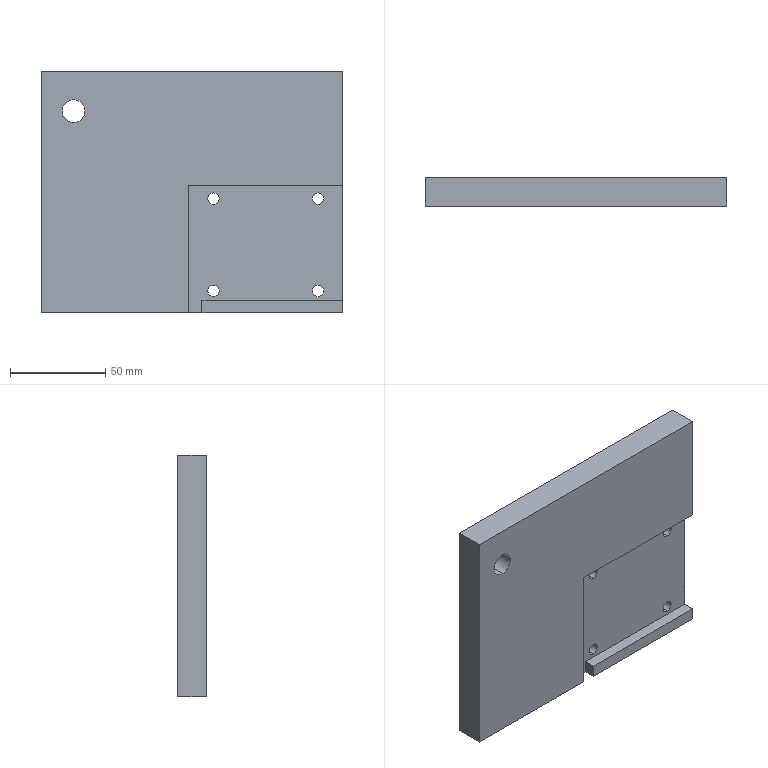Part | SolidWorks | features ICE 6, Extrusion 1, HoleWzd 1 | 1 solid | 34 faces | box 158.5 x 15 x 127 mm | volume 237591 mm3 | plane 16 | cylinder 14 | cone 4 | commonest cylinder face diameters 6 x8 5 x2 12 x2 20 x2
STEP:
#1=CARTESIAN_POINT('',(-38.25,9.498,24.5));
#2=VERTEX_POINT('',#1);
#3=CARTESIAN_POINT('',(-38.25,11.,27.));
#4=VERTEX_POINT('',#3);
#5=CARTESIAN_POINT('',(-38.25,11.,27.));
#6=DIRECTION('',(0.,0.515,0.8572));
#7=VECTOR('',#6,1000.);
#8=LINE('',#5,#7);
#9=EDGE_CURVE('',#2,#4,#8,.T.);
#10=ORIENTED_EDGE('',*,*,#9,.F.);
#11=CARTESIAN_POINT('',(-38.25,11.,22.));
#12=VERTEX_POINT('',#11);
#13=CARTESIAN_POINT('',(-38.25,11.,22.));
#14=DIRECTION('',(0.,0.515,-0.8572));
#15=VECTOR('',#14,1000.);
#16=LINE('',#13,#15);
#17=EDGE_CURVE('',#2,#12,#16,.T.);
#18=ORIENTED_EDGE('',*,*,#17,.T.);
#19=CARTESIAN_POINT('',(-38.25,11.,24.5));
#20=DIRECTION('',(0.,1.,0.));
#21=DIRECTION('',(0.,0.,1.));
#22=AXIS2_PLACEMENT_3D('',#19,#20,#21);
#23=CIRCLE('',#22,2.5);
#24=EDGE_CURVE('',#12,#4,#23,.T.);
#25=ORIENTED_EDGE('',*,*,#24,.T.);
#26=EDGE_LOOP('',(#10,#18,#25));
#27=FACE_OUTER_BOUND('',#26,.T.);
#28=CARTESIAN_POINT('',(-38.25,11.,24.5));
#29=DIRECTION('',(0.,1.,0.));
#30=DIRECTION('',(0.,0.,1.));
#31=AXIS2_PLACEMENT_3D('',#28,#29,#30);
#32=CONICAL_SURFACE('',#31,2.5,1.03);
#33=ADVANCED_FACE('',(#27),#32,.F.);
#34=CARTESIAN_POINT('',(-38.25,14.975,27.));
#35=VERTEX_POINT('',#34);
#36=CARTESIAN_POINT('',(-35.75,14.975,24.5));
#37=VERTEX_POINT('',#36);
#38=CARTESIAN_POINT('',(-38.25,14.975,24.5));
#39=DIRECTION('',(0.,1.,0.));
#40=DIRECTION('',(0.,0.,1.));
#41=AXIS2_PLACEMENT_3D('',#38,#39,#40);
#42=CIRCLE('',#41,2.5);
#43=EDGE_CURVE('',#35,#37,#42,.T.);
#44=ORIENTED_EDGE('',*,*,#43,.F.);
#45=CARTESIAN_POINT('',(-38.25,15.,27.025));
#46=VERTEX_POINT('',#45);
#47=CARTESIAN_POINT('',(-38.25,15.,27.025));
#48=DIRECTION('',(0.,0.7071,0.7071));
#49=VECTOR('',#48,1000.);
#50=LINE('',#47,#49);
#51=EDGE_CURVE('',#35,#46,#50,.T.);
#52=ORIENTED_EDGE('',*,*,#51,.T.);
#53=CARTESIAN_POINT('',(-35.725,15.,24.5));
#54=VERTEX_POINT('',#53);
#55=CARTESIAN_POINT('',(-38.25,15.,24.5));
#56=DIRECTION('',(0.,1.,0.));
#57=DIRECTION('',(0.,0.,1.));
#58=AXIS2_PLACEMENT_3D('',#55,#56,#57);
#59=CIRCLE('',#58,2.525);
#60=EDGE_CURVE('',#46,#54,#59,.T.);
#61=ORIENTED_EDGE('',*,*,#60,.T.);
#62=CARTESIAN_POINT('',(-38.25,12.475,24.5));
#63=DIRECTION('',(0.7071,0.7071,0.));
#64=VECTOR('',#63,1000.);
#65=LINE('',#62,#64);
#66=EDGE_CURVE('',#37,#54,#65,.T.);
#67=ORIENTED_EDGE('',*,*,#66,.F.);
#68=EDGE_LOOP('',(#44,#52,#61,#67));
#69=FACE_OUTER_BOUND('',#68,.T.);
#70=CARTESIAN_POINT('',(-38.25,15.,24.5));
#71=DIRECTION('',(0.,1.,0.));
#72=DIRECTION('',(0.,0.,1.));
#73=AXIS2_PLACEMENT_3D('',#70,#71,#72);
#74=CONICAL_SURFACE('',#73,2.525,0.7854);
#75=ADVANCED_FACE('',(#69),#74,.F.);
#76=ORIENTED_EDGE('',*,*,#24,.F.);
#77=CARTESIAN_POINT('',(-38.25,12.,22.));
#78=VERTEX_POINT('',#77);
#79=CARTESIAN_POINT('',(-38.25,15.,22.));
#80=DIRECTION('',(0.,1.,0.));
#81=VECTOR('',#80,1000.);
#82=LINE('',#79,#81);
#83=EDGE_CURVE('',#12,#78,#82,.T.);
#84=ORIENTED_EDGE('',*,*,#83,.T.);
#85=CARTESIAN_POINT('',(-38.25,14.975,22.));
#86=VERTEX_POINT('',#85);
#87=CARTESIAN_POINT('',(-38.25,15.,22.));
#88=DIRECTION('',(0.,-1.,0.));
#89=VECTOR('',#88,1000.);
#90=LINE('',#87,#89);
#91=EDGE_CURVE('',#86,#78,#90,.T.);
#92=ORIENTED_EDGE('',*,*,#91,.F.);
#93=CARTESIAN_POINT('',(-38.25,14.975,24.5));
#94=DIRECTION('',(0.,1.,0.));
#95=DIRECTION('',(0.,0.,1.));
#96=AXIS2_PLACEMENT_3D('',#93,#94,#95);
#97=CIRCLE('',#96,2.5);
#98=EDGE_CURVE('',#86,#35,#97,.T.);
#99=ORIENTED_EDGE('',*,*,#98,.T.);
#100=CARTESIAN_POINT('',(-38.25,15.,27.));
#101=DIRECTION('',(0.,1.,0.));
#102=VECTOR('',#101,1000.);
#103=LINE('',#100,#102);
#104=EDGE_CURVE('',#4,#35,#103,.T.);
#105=ORIENTED_EDGE('',*,*,#104,.F.);
#106=EDGE_LOOP('',(#76,#84,#92,#99,#105));
#107=FACE_OUTER_BOUND('',#106,.T.);
#108=CARTESIAN_POINT('',(-38.25,15.,24.5));
#109=DIRECTION('',(0.,1.,0.));
#110=DIRECTION('',(0.,0.,1.));
#111=AXIS2_PLACEMENT_3D('',#108,#109,#110);
#112=CYLINDRICAL_SURFACE('',#111,2.5);
#113=ADVANCED_FACE('',(#107),#112,.F.);
#114=CARTESIAN_POINT('',(-62.25,0.,36.5));
#115=VERTEX_POINT('',#114);
#116=CARTESIAN_POINT('',(-62.25,0.,48.5));
#117=VERTEX_POINT('',#116);
#118=CARTESIAN_POINT('',(-62.25,0.,42.5));
#119=DIRECTION('',(0.,1.,0.));
#120=DIRECTION('',(0.,0.,1.));
#121=AXIS2_PLACEMENT_3D('',#118,#119,#120);
#122=CIRCLE('',#121,6.);
#123=EDGE_CURVE('',#115,#117,#122,.T.);
#124=ORIENTED_EDGE('',*,*,#123,.F.);
#125=CARTESIAN_POINT('',(-62.25,9.,36.5));
#126=VERTEX_POINT('',#125);
#127=CARTESIAN_POINT('',(-62.25,0.,36.5));
#128=DIRECTION('',(0.,1.,0.));
#129=VECTOR('',#128,1000.);
#130=LINE('',#127,#129);
#131=EDGE_CURVE('',#115,#126,#130,.T.);
#132=ORIENTED_EDGE('',*,*,#131,.T.);
#133=CARTESIAN_POINT('',(-62.25,9.,48.5));
#134=VERTEX_POINT('',#133);
#135=CARTESIAN_POINT('',(-62.25,9.,42.5));
#136=DIRECTION('',(0.,1.,0.));
#137=DIRECTION('',(0.,0.,1.));
#138=AXIS2_PLACEMENT_3D('',#135,#136,#137);
#139=CIRCLE('',#138,6.);
#140=EDGE_CURVE('',#126,#134,#139,.T.);
#141=ORIENTED_EDGE('',*,*,#140,.T.);
#142=CARTESIAN_POINT('',(-62.25,0.,48.5));
#143=DIRECTION('',(0.,1.,0.));
#144=VECTOR('',#143,1000.);
#145=LINE('',#142,#144);
#146=EDGE_CURVE('',#117,#134,#145,.T.);
#147=ORIENTED_EDGE('',*,*,#146,.F.);
#148=EDGE_LOOP('',(#124,#132,#141,#147));
#149=FACE_OUTER_BOUND('',#148,.T.);
#150=CARTESIAN_POINT('',(-62.25,0.,42.5));
#151=DIRECTION('',(0.,1.,0.));
#152=DIRECTION('',(0.,0.,1.));
#153=AXIS2_PLACEMENT_3D('',#150,#151,#152);
#154=CYLINDRICAL_SURFACE('',#153,6.);
#155=ADVANCED_FACE('',(#149),#154,.F.);
#156=CARTESIAN_POINT('',(-62.25,9.,32.5));
#157=VERTEX_POINT('',#156);
#158=CARTESIAN_POINT('',(-62.25,9.,52.5));
#159=VERTEX_POINT('',#158);
#160=CARTESIAN_POINT('',(-62.25,9.,42.5));
#161=DIRECTION('',(0.,1.,0.));
#162=DIRECTION('',(0.,0.,1.));
#163=AXIS2_PLACEMENT_3D('',#160,#161,#162);
#164=CIRCLE('',#163,10.);
#165=EDGE_CURVE('',#157,#159,#164,.T.);
#166=ORIENTED_EDGE('',*,*,#165,.F.);
#167=CARTESIAN_POINT('',(-62.25,15.,32.5));
#168=VERTEX_POINT('',#167);
#169=CARTESIAN_POINT('',(-62.25,9.,32.5));
#170=DIRECTION('',(0.,1.,0.));
#171=VECTOR('',#170,1000.);
#172=LINE('',#169,#171);
#173=EDGE_CURVE('',#157,#168,#172,.T.);
#174=ORIENTED_EDGE('',*,*,#173,.T.);
#175=CARTESIAN_POINT('',(-62.25,15.,52.5));
#176=VERTEX_POINT('',#175);
#177=CARTESIAN_POINT('',(-62.25,15.,42.5));
#178=DIRECTION('',(0.,1.,0.));
#179=DIRECTION('',(0.,0.,1.));
#180=AXIS2_PLACEMENT_3D('',#177,#178,#179);
#181=CIRCLE('',#180,10.);
#182=EDGE_CURVE('',#168,#176,#181,.T.);
#183=ORIENTED_EDGE('',*,*,#182,.T.);
#184=CARTESIAN_POINT('',(-62.25,9.,52.5));
#185=DIRECTION('',(0.,1.,0.));
#186=VECTOR('',#185,1000.);
#187=LINE('',#184,#186);
#188=EDGE_CURVE('',#159,#176,#187,.T.);
#189=ORIENTED_EDGE('',*,*,#188,.F.);
#190=EDGE_LOOP('',(#166,#174,#183,#189));
#191=FACE_OUTER_BOUND('',#190,.T.);
#192=CARTESIAN_POINT('',(-62.25,9.,42.5));
#193=DIRECTION('',(0.,1.,0.));
#194=DIRECTION('',(0.,0.,1.));
#195=AXIS2_PLACEMENT_3D('',#192,#193,#194);
#196=CYLINDRICAL_SURFACE('',#195,10.);
#197=ADVANCED_FACE('',(#191),#196,.F.);
#198=CARTESIAN_POINT('',(11.25,6.,-0.5));
#199=VERTEX_POINT('',#198);
#200=CARTESIAN_POINT('',(11.25,6.,-6.5));
#201=VERTEX_POINT('',#200);
#202=CARTESIAN_POINT('',(11.25,6.,-3.5));
#203=DIRECTION('',(0.,-1.,0.));
#204=DIRECTION('',(0.,0.,-1.));
#205=AXIS2_PLACEMENT_3D('',#202,#203,#204);
#206=CIRCLE('',#205,3.);
#207=EDGE_CURVE('',#199,#201,#206,.T.);
#208=ORIENTED_EDGE('',*,*,#207,.T.);
#209=CARTESIAN_POINT('',(11.25,12.,-6.5));
#210=VERTEX_POINT('',#209);
#211=CARTESIAN_POINT('',(11.25,0.,-6.5));
#212=DIRECTION('',(0.,1.,0.));
#213=VECTOR('',#212,1000.);
#214=LINE('',#211,#213);
#215=EDGE_CURVE('',#201,#210,#214,.T.);
#216=ORIENTED_EDGE('',*,*,#215,.T.);
#217=CARTESIAN_POINT('',(11.25,12.,-0.5));
#218=VERTEX_POINT('',#217);
#219=CARTESIAN_POINT('',(11.25,12.,-3.5));
#220=DIRECTION('',(0.,-1.,0.));
#221=DIRECTION('',(0.,0.,-1.));
#222=AXIS2_PLACEMENT_3D('',#219,#220,#221);
#223=CIRCLE('',#222,3.);
#224=EDGE_CURVE('',#218,#210,#223,.T.);
#225=ORIENTED_EDGE('',*,*,#224,.F.);
#226=CARTESIAN_POINT('',(11.25,0.,-0.5));
#227=DIRECTION('',(0.,1.,0.));
#228=VECTOR('',#227,1000.);
#229=LINE('',#226,#228);
#230=EDGE_CURVE('',#199,#218,#229,.T.);
#231=ORIENTED_EDGE('',*,*,#230,.F.);
#232=EDGE_LOOP('',(#208,#216,#225,#231));
#233=FACE_OUTER_BOUND('',#232,.T.);
#234=CARTESIAN_POINT('',(11.25,0.,-3.5));
#235=DIRECTION('',(0.,1.,0.));
#236=DIRECTION('',(0.,0.,1.));
#237=AXIS2_PLACEMENT_3D('',#234,#235,#236);
#238=CYLINDRICAL_SURFACE('',#237,3.);
#239=ADVANCED_FACE('',(#233),#238,.F.);
#240=CARTESIAN_POINT('',(66.25,6.,-0.5));
#241=VERTEX_POINT('',#240);
#242=CARTESIAN_POINT('',(66.25,6.,-6.5));
#243=VERTEX_POINT('',#242);
#244=CARTESIAN_POINT('',(66.25,6.,-3.5));
#245=DIRECTION('',(0.,-1.,0.));
#246=DIRECTION('',(0.,0.,-1.));
#247=AXIS2_PLACEMENT_3D('',#244,#245,#246);
#248=CIRCLE('',#247,3.);
#249=EDGE_CURVE('',#241,#243,#248,.T.);
#250=ORIENTED_EDGE('',*,*,#249,.T.);
#251=CARTESIAN_POINT('',(66.25,12.,-6.5));
#252=VERTEX_POINT('',#251);
#253=CARTESIAN_POINT('',(66.25,0.,-6.5));
#254=DIRECTION('',(0.,1.,0.));
#255=VECTOR('',#254,1000.);
#256=LINE('',#253,#255);
#257=EDGE_CURVE('',#243,#252,#256,.T.);
#258=ORIENTED_EDGE('',*,*,#257,.T.);
#259=CARTESIAN_POINT('',(66.25,12.,-0.5));
#260=VERTEX_POINT('',#259);
#261=CARTESIAN_POINT('',(66.25,12.,-3.5));
#262=DIRECTION('',(0.,-1.,0.));
#263=DIRECTION('',(0.,0.,-1.));
#264=AXIS2_PLACEMENT_3D('',#261,#262,#263);
#265=CIRCLE('',#264,3.);
#266=EDGE_CURVE('',#260,#252,#265,.T.);
#267=ORIENTED_EDGE('',*,*,#266,.F.);
#268=CARTESIAN_POINT('',(66.25,0.,-0.5));
#269=DIRECTION('',(0.,1.,0.));
#270=VECTOR('',#269,1000.);
#271=LINE('',#268,#270);
#272=EDGE_CURVE('',#241,#260,#271,.T.);
#273=ORIENTED_EDGE('',*,*,#272,.F.);
#274=EDGE_LOOP('',(#250,#258,#267,#273));
#275=FACE_OUTER_BOUND('',#274,.T.);
#276=CARTESIAN_POINT('',(66.25,0.,-3.5));
#277=DIRECTION('',(0.,1.,0.));
#278=DIRECTION('',(0.,0.,1.));
#279=AXIS2_PLACEMENT_3D('',#276,#277,#278);
#280=CYLINDRICAL_SURFACE('',#279,3.);
#281=ADVANCED_FACE('',(#275),#280,.F.);
#282=CARTESIAN_POINT('',(66.25,6.,-49.));
#283=VERTEX_POINT('',#282);
#284=CARTESIAN_POINT('',(66.25,6.,-55.));
#285=VERTEX_POINT('',#284);
#286=CARTESIAN_POINT('',(66.25,6.,-52.));
#287=DIRECTION('',(0.,-1.,0.));
#288=DIRECTION('',(0.,0.,-1.));
#289=AXIS2_PLACEMENT_3D('',#286,#287,#288);
#290=CIRCLE('',#289,3.);
#291=EDGE_CURVE('',#283,#285,#290,.T.);
#292=ORIENTED_EDGE('',*,*,#291,.T.);
#293=CARTESIAN_POINT('',(66.25,12.,-55.));
#294=VERTEX_POINT('',#293);
#295=CARTESIAN_POINT('',(66.25,0.,-55.));
#296=DIRECTION('',(0.,1.,0.));
#297=VECTOR('',#296,1000.);
#298=LINE('',#295,#297);
#299=EDGE_CURVE('',#285,#294,#298,.T.);
#300=ORIENTED_EDGE('',*,*,#299,.T.);
#301=CARTESIAN_POINT('',(66.25,12.,-49.));
#302=VERTEX_POINT('',#301);
#303=CARTESIAN_POINT('',(66.25,12.,-52.));
#304=DIRECTION('',(0.,-1.,0.));
#305=DIRECTION('',(0.,0.,-1.));
#306=AXIS2_PLACEMENT_3D('',#303,#304,#305);
#307=CIRCLE('',#306,3.);
#308=EDGE_CURVE('',#302,#294,#307,.T.);
#309=ORIENTED_EDGE('',*,*,#308,.F.);
#310=CARTESIAN_POINT('',(66.25,0.,-49.));
#311=DIRECTION('',(0.,1.,0.));
#312=VECTOR('',#311,1000.);
#313=LINE('',#310,#312);
#314=EDGE_CURVE('',#283,#302,#313,.T.);
#315=ORIENTED_EDGE('',*,*,#314,.F.);
#316=EDGE_LOOP('',(#292,#300,#309,#315));
#317=FACE_OUTER_BOUND('',#316,.T.);
#318=CARTESIAN_POINT('',(66.25,0.,-52.));
#319=DIRECTION('',(0.,1.,0.));
#320=DIRECTION('',(0.,0.,1.));
#321=AXIS2_PLACEMENT_3D('',#318,#319,#320);
#322=CYLINDRICAL_SURFACE('',#321,3.);
#323=ADVANCED_FACE('',(#317),#322,.F.);
#324=CARTESIAN_POINT('',(11.25,6.,-49.));
#325=VERTEX_POINT('',#324);
#326=CARTESIAN_POINT('',(11.25,6.,-55.));
#327=VERTEX_POINT('',#326);
#328=CARTESIAN_POINT('',(11.25,6.,-52.));
#329=DIRECTION('',(0.,-1.,0.));
#330=DIRECTION('',(0.,0.,-1.));
#331=AXIS2_PLACEMENT_3D('',#328,#329,#330);
#332=CIRCLE('',#331,3.);
#333=EDGE_CURVE('',#325,#327,#332,.T.);
#334=ORIENTED_EDGE('',*,*,#333,.T.);
#335=CARTESIAN_POINT('',(11.25,12.,-55.));
#336=VERTEX_POINT('',#335);
#337=CARTESIAN_POINT('',(11.25,0.,-55.));
#338=DIRECTION('',(0.,1.,0.));
#339=VECTOR('',#338,1000.);
#340=LINE('',#337,#339);
#341=EDGE_CURVE('',#327,#336,#340,.T.);
#342=ORIENTED_EDGE('',*,*,#341,.T.);
#343=CARTESIAN_POINT('',(11.25,12.,-49.));
#344=VERTEX_POINT('',#343);
#345=CARTESIAN_POINT('',(11.25,12.,-52.));
#346=DIRECTION('',(0.,-1.,0.));
#347=DIRECTION('',(0.,0.,-1.));
#348=AXIS2_PLACEMENT_3D('',#345,#346,#347);
#349=CIRCLE('',#348,3.);
#350=EDGE_CURVE('',#344,#336,#349,.T.);
#351=ORIENTED_EDGE('',*,*,#350,.F.);
#352=CARTESIAN_POINT('',(11.25,0.,-49.));
#353=DIRECTION('',(0.,1.,0.));
#354=VECTOR('',#353,1000.);
#355=LINE('',#352,#354);
#356=EDGE_CURVE('',#325,#344,#355,.T.);
#357=ORIENTED_EDGE('',*,*,#356,.F.);
#358=EDGE_LOOP('',(#334,#342,#351,#357));
#359=FACE_OUTER_BOUND('',#358,.T.);
#360=CARTESIAN_POINT('',(11.25,0.,-52.));
#361=DIRECTION('',(0.,1.,0.));
#362=DIRECTION('',(0.,0.,1.));
#363=AXIS2_PLACEMENT_3D('',#360,#361,#362);
#364=CYLINDRICAL_SURFACE('',#363,3.);
#365=ADVANCED_FACE('',(#359),#364,.F.);
#366=CARTESIAN_POINT('',(-62.25,0.,42.5));
#367=DIRECTION('',(0.,1.,0.));
#368=DIRECTION('',(0.,0.,1.));
#369=AXIS2_PLACEMENT_3D('',#366,#367,#368);
#370=CIRCLE('',#369,6.);
#371=EDGE_CURVE('',#117,#115,#370,.T.);
#372=ORIENTED_EDGE('',*,*,#371,.T.);
#373=ORIENTED_EDGE('',*,*,#123,.T.);
#374=EDGE_LOOP('',(#372,#373));
#375=FACE_BOUND('',#374,.T.);
#376=CARTESIAN_POINT('',(-1.75,0.,-63.5));
#377=VERTEX_POINT('',#376);
#378=CARTESIAN_POINT('',(-79.25,0.,-63.5));
#379=VERTEX_POINT('',#378);
#380=CARTESIAN_POINT('',(-79.25,0.,-63.5));
#381=DIRECTION('',(-1.,0.,0.));
#382=VECTOR('',#381,1000.);
#383=LINE('',#380,#382);
#384=EDGE_CURVE('',#377,#379,#383,.T.);
#385=ORIENTED_EDGE('',*,*,#384,.F.);
#386=CARTESIAN_POINT('',(-1.75,0.,3.5));
#387=VERTEX_POINT('',#386);
#388=CARTESIAN_POINT('',(-1.75,0.,-57.));
#389=DIRECTION('',(0.,0.,-1.));
#390=VECTOR('',#389,1000.);
#391=LINE('',#388,#390);
#392=EDGE_CURVE('',#387,#377,#391,.T.);
#393=ORIENTED_EDGE('',*,*,#392,.F.);
#394=CARTESIAN_POINT('',(79.25,0.,3.5));
#395=VERTEX_POINT('',#394);
#396=CARTESIAN_POINT('',(79.25,0.,3.5));
#397=DIRECTION('',(-1.,0.,0.));
#398=VECTOR('',#397,1000.);
#399=LINE('',#396,#398);
#400=EDGE_CURVE('',#395,#387,#399,.T.);
#401=ORIENTED_EDGE('',*,*,#400,.F.);
#402=CARTESIAN_POINT('',(79.25,0.,63.5));
#403=VERTEX_POINT('',#402);
#404=CARTESIAN_POINT('',(79.25,0.,-63.5));
#405=DIRECTION('',(0.,0.,-1.));
#406=VECTOR('',#405,1000.);
#407=LINE('',#404,#406);
#408=EDGE_CURVE('',#403,#395,#407,.T.);
#409=ORIENTED_EDGE('',*,*,#408,.F.);
#410=CARTESIAN_POINT('',(-79.25,0.,63.5));
#411=VERTEX_POINT('',#410);
#412=CARTESIAN_POINT('',(-79.25,0.,63.5));
#413=DIRECTION('',(1.,0.,0.));
#414=VECTOR('',#413,1000.);
#415=LINE('',#412,#414);
#416=EDGE_CURVE('',#411,#403,#415,.T.);
#417=ORIENTED_EDGE('',*,*,#416,.F.);
#418=CARTESIAN_POINT('',(-79.25,0.,-63.5));
#419=DIRECTION('',(0.,0.,1.));
#420=VECTOR('',#419,1000.);
#421=LINE('',#418,#420);
#422=EDGE_CURVE('',#379,#411,#421,.T.);
#423=ORIENTED_EDGE('',*,*,#422,.F.);
#424=EDGE_LOOP('',(#385,#393,#401,#409,#417,#423));
#425=FACE_OUTER_BOUND('',#424,.T.);
#426=CARTESIAN_POINT('',(0.,0.,0.));
#427=DIRECTION('',(0.,1.,0.));
#428=DIRECTION('',(0.,0.,1.));
#429=AXIS2_PLACEMENT_3D('',#426,#427,#428);
#430=PLANE('',#429);
#431=ADVANCED_FACE('',(#375,#425),#430,.F.);
#432=CARTESIAN_POINT('',(79.25,6.,-57.));
#433=VERTEX_POINT('',#432);
#434=CARTESIAN_POINT('',(79.25,6.,3.5));
#435=VERTEX_POINT('',#434);
#436=CARTESIAN_POINT('',(79.25,6.,-57.));
#437=DIRECTION('',(0.,0.,1.));
#438=VECTOR('',#437,1000.);
#439=LINE('',#436,#438);
#440=EDGE_CURVE('',#433,#435,#439,.T.);
#441=ORIENTED_EDGE('',*,*,#440,.F.);
#442=CARTESIAN_POINT('',(79.25,0.,-57.));
#443=VERTEX_POINT('',#442);
#444=CARTESIAN_POINT('',(79.25,6.,-57.));
#445=DIRECTION('',(0.,-1.,0.));
#446=VECTOR('',#445,1000.);
#447=LINE('',#444,#446);
#448=EDGE_CURVE('',#433,#443,#447,.T.);
#449=ORIENTED_EDGE('',*,*,#448,.T.);
#450=CARTESIAN_POINT('',(79.25,0.,-63.5));
#451=VERTEX_POINT('',#450);
#452=CARTESIAN_POINT('',(79.25,0.,-63.5));
#453=DIRECTION('',(0.,0.,-1.));
#454=VECTOR('',#453,1000.);
#455=LINE('',#452,#454);
#456=EDGE_CURVE('',#443,#451,#455,.T.);
#457=ORIENTED_EDGE('',*,*,#456,.T.);
#458=CARTESIAN_POINT('',(79.25,12.,-63.5));
#459=VERTEX_POINT('',#458);
#460=CARTESIAN_POINT('',(79.25,15.,-63.5));
#461=DIRECTION('',(0.,-1.,0.));
#462=VECTOR('',#461,1000.);
#463=LINE('',#460,#462);
#464=EDGE_CURVE('',#459,#451,#463,.T.);
#465=ORIENTED_EDGE('',*,*,#464,.F.);
#466=CARTESIAN_POINT('',(79.25,12.,24.5));
#467=VERTEX_POINT('',#466);
#468=CARTESIAN_POINT('',(79.25,12.,-63.5));
#469=DIRECTION('',(0.,0.,-1.));
#470=VECTOR('',#469,1000.);
#471=LINE('',#468,#470);
#472=EDGE_CURVE('',#467,#459,#471,.T.);
#473=ORIENTED_EDGE('',*,*,#472,.F.);
#474=CARTESIAN_POINT('',(79.25,15.,24.5));
#475=VERTEX_POINT('',#474);
#476=CARTESIAN_POINT('',(79.25,12.,24.5));
#477=DIRECTION('',(0.,1.,0.));
#478=VECTOR('',#477,1000.);
#479=LINE('',#476,#478);
#480=EDGE_CURVE('',#467,#475,#479,.T.);
#481=ORIENTED_EDGE('',*,*,#480,.T.);
#482=CARTESIAN_POINT('',(79.25,15.,63.5));
#483=VERTEX_POINT('',#482);
#484=CARTESIAN_POINT('',(79.25,15.,-63.5));
#485=DIRECTION('',(0.,0.,-1.));
#486=VECTOR('',#485,1000.);
#487=LINE('',#484,#486);
#488=EDGE_CURVE('',#483,#475,#487,.T.);
#489=ORIENTED_EDGE('',*,*,#488,.F.);
#490=CARTESIAN_POINT('',(79.25,15.,63.5));
#491=DIRECTION('',(0.,-1.,0.));
#492=VECTOR('',#491,1000.);
#493=LINE('',#490,#492);
#494=EDGE_CURVE('',#483,#403,#493,.T.);
#495=ORIENTED_EDGE('',*,*,#494,.T.);
#496=ORIENTED_EDGE('',*,*,#408,.T.);
#497=CARTESIAN_POINT('',(79.25,6.,3.5));
#498=DIRECTION('',(0.,-1.,0.));
#499=VECTOR('',#498,1000.);
#500=LINE('',#497,#499);
#501=EDGE_CURVE('',#435,#395,#500,.T.);
#502=ORIENTED_EDGE('',*,*,#501,.F.);
#503=EDGE_LOOP('',(#441,#449,#457,#465,#473,#481,#489,#495,#496,#502));
#504=FACE_OUTER_BOUND('',#503,.T.);
#505=CARTESIAN_POINT('',(79.25,15.,-63.5));
#506=DIRECTION('',(-1.,0.,0.));
#507=DIRECTION('',(0.,0.,1.));
#508=AXIS2_PLACEMENT_3D('',#505,#506,#507);
#509=PLANE('',#508);
#510=ADVANCED_FACE('',(#504),#509,.F.);
#511=CARTESIAN_POINT('',(5.25,6.,-63.5));
#512=VERTEX_POINT('',#511);
#513=CARTESIAN_POINT('',(-1.75,6.,-63.5));
#514=VERTEX_POINT('',#513);
#515=CARTESIAN_POINT('',(-1.75,6.,-63.5));
#516=DIRECTION('',(-1.,0.,0.));
#517=VECTOR('',#516,1000.);
#518=LINE('',#515,#517);
#519=EDGE_CURVE('',#512,#514,#518,.T.);
#520=ORIENTED_EDGE('',*,*,#519,.T.);
#521=CARTESIAN_POINT('',(-1.75,0.,-63.5));
#522=DIRECTION('',(0.,-1.,0.));
#523=VECTOR('',#522,1000.);
#524=LINE('',#521,#523);
#525=EDGE_CURVE('',#514,#377,#524,.T.);
#526=ORIENTED_EDGE('',*,*,#525,.T.);
#527=ORIENTED_EDGE('',*,*,#384,.T.);
#528=CARTESIAN_POINT('',(-79.25,15.,-63.5));
#529=VERTEX_POINT('',#528);
#530=CARTESIAN_POINT('',(-79.25,15.,-63.5));
#531=DIRECTION('',(0.,-1.,0.));
#532=VECTOR('',#531,1000.);
#533=LINE('',#530,#532);
#534=EDGE_CURVE('',#529,#379,#533,.T.);
#535=ORIENTED_EDGE('',*,*,#534,.F.);
#536=CARTESIAN_POINT('',(-38.25,15.,-63.5));
#537=VERTEX_POINT('',#536);
#538=CARTESIAN_POINT('',(-79.25,15.,-63.5));
#539=DIRECTION('',(-1.,0.,0.));
#540=VECTOR('',#539,1000.);
#541=LINE('',#538,#540);
#542=EDGE_CURVE('',#537,#529,#541,.T.);
#543=ORIENTED_EDGE('',*,*,#542,.F.);
#544=CARTESIAN_POINT('',(-38.25,12.,-63.5));
#545=VERTEX_POINT('',#544);
#546=CARTESIAN_POINT('',(-38.25,12.,-63.5));
#547=DIRECTION('',(0.,1.,0.));
#548=VECTOR('',#547,1000.);
#549=LINE('',#546,#548);
#550=EDGE_CURVE('',#545,#537,#549,.T.);
#551=ORIENTED_EDGE('',*,*,#550,.F.);
#552=CARTESIAN_POINT('',(79.25,12.,-63.5));
#553=DIRECTION('',(-1.,0.,0.));
#554=VECTOR('',#553,1000.);
#555=LINE('',#552,#554);
#556=EDGE_CURVE('',#459,#545,#555,.T.);
#557=ORIENTED_EDGE('',*,*,#556,.F.);
#558=ORIENTED_EDGE('',*,*,#464,.T.);
#559=CARTESIAN_POINT('',(5.25,0.,-63.5));
#560=VERTEX_POINT('',#559);
#561=CARTESIAN_POINT('',(-79.25,0.,-63.5));
#562=DIRECTION('',(-1.,0.,0.));
#563=VECTOR('',#562,1000.);
#564=LINE('',#561,#563);
#565=EDGE_CURVE('',#451,#560,#564,.T.);
#566=ORIENTED_EDGE('',*,*,#565,.T.);
#567=CARTESIAN_POINT('',(5.25,0.,-63.5));
#568=DIRECTION('',(0.,1.,0.));
#569=VECTOR('',#568,1000.);
#570=LINE('',#567,#569);
#571=EDGE_CURVE('',#560,#512,#570,.T.);
#572=ORIENTED_EDGE('',*,*,#571,.T.);
#573=EDGE_LOOP('',(#520,#526,#527,#535,#543,#551,#557,#558,#566,#572));
#574=FACE_OUTER_BOUND('',#573,.T.);
#575=CARTESIAN_POINT('',(-79.25,15.,-63.5));
#576=DIRECTION('',(0.,0.,1.));
#577=DIRECTION('',(1.,0.,0.));
#578=AXIS2_PLACEMENT_3D('',#575,#576,#577);
#579=PLANE('',#578);
#580=ADVANCED_FACE('',(#574),#579,.F.);
#581=ORIENTED_EDGE('',*,*,#422,.T.);
#582=CARTESIAN_POINT('',(-79.25,15.,63.5));
#583=VERTEX_POINT('',#582);
#584=CARTESIAN_POINT('',(-79.25,15.,63.5));
#585=DIRECTION('',(0.,-1.,0.));
#586=VECTOR('',#585,1000.);
#587=LINE('',#584,#586);
#588=EDGE_CURVE('',#583,#411,#587,.T.);
#589=ORIENTED_EDGE('',*,*,#588,.F.);
#590=CARTESIAN_POINT('',(-79.25,15.,-63.5));
#591=DIRECTION('',(0.,0.,1.));
#592=VECTOR('',#591,1000.);
#593=LINE('',#590,#592);
#594=EDGE_CURVE('',#529,#583,#593,.T.);
#595=ORIENTED_EDGE('',*,*,#594,.F.);
#596=ORIENTED_EDGE('',*,*,#534,.T.);
#597=EDGE_LOOP('',(#581,#589,#595,#596));
#598=FACE_OUTER_BOUND('',#597,.T.);
#599=CARTESIAN_POINT('',(-79.25,15.,-63.5));
#600=DIRECTION('',(1.,0.,0.));
#601=DIRECTION('',(0.,0.,-1.));
#602=AXIS2_PLACEMENT_3D('',#599,#600,#601);
#603=PLANE('',#602);
#604=ADVANCED_FACE('',(#598),#603,.F.);
#605=ORIENTED_EDGE('',*,*,#416,.T.);
#606=ORIENTED_EDGE('',*,*,#494,.F.);
#607=CARTESIAN_POINT('',(-79.25,15.,63.5));
#608=DIRECTION('',(1.,0.,0.));
#609=VECTOR('',#608,1000.);
#610=LINE('',#607,#609);
#611=EDGE_CURVE('',#583,#483,#610,.T.);
#612=ORIENTED_EDGE('',*,*,#611,.F.);
#613=ORIENTED_EDGE('',*,*,#588,.T.);
#614=EDGE_LOOP('',(#605,#606,#612,#613));
#615=FACE_OUTER_BOUND('',#614,.T.);
#616=CARTESIAN_POINT('',(-79.25,15.,63.5));
#617=DIRECTION('',(0.,0.,-1.));
#618=DIRECTION('',(-1.,0.,0.));
#619=AXIS2_PLACEMENT_3D('',#616,#617,#618);
#620=PLANE('',#619);
#621=ADVANCED_FACE('',(#615),#620,.F.);
#622=CARTESIAN_POINT('',(-38.25,15.,21.975));
#623=VERTEX_POINT('',#622);
#624=CARTESIAN_POINT('',(-38.25,15.,24.5));
#625=DIRECTION('',(0.,1.,0.));
#626=DIRECTION('',(0.,0.,1.));
#627=AXIS2_PLACEMENT_3D('',#624,#625,#626);
#628=CIRCLE('',#627,2.525);
#629=EDGE_CURVE('',#623,#46,#628,.T.);
#630=ORIENTED_EDGE('',*,*,#629,.F.);
#631=CARTESIAN_POINT('',(-38.25,15.,-63.5));
#632=DIRECTION('',(0.,0.,1.));
#633=VECTOR('',#632,1000.);
#634=LINE('',#631,#633);
#635=EDGE_CURVE('',#537,#623,#634,.T.);
#636=ORIENTED_EDGE('',*,*,#635,.F.);
#637=ORIENTED_EDGE('',*,*,#542,.T.);
#638=ORIENTED_EDGE('',*,*,#594,.T.);
#639=ORIENTED_EDGE('',*,*,#611,.T.);
#640=ORIENTED_EDGE('',*,*,#488,.T.);
#641=CARTESIAN_POINT('',(79.25,15.,24.5));
#642=DIRECTION('',(1.,0.,0.));
#643=VECTOR('',#642,1000.);
#644=LINE('',#641,#643);
#645=EDGE_CURVE('',#54,#475,#644,.T.);
#646=ORIENTED_EDGE('',*,*,#645,.F.);
#647=ORIENTED_EDGE('',*,*,#60,.F.);
#648=EDGE_LOOP('',(#630,#636,#637,#638,#639,#640,#646,#647));
#649=FACE_OUTER_BOUND('',#648,.T.);
#650=CARTESIAN_POINT('',(-62.25,15.,42.5));
#651=DIRECTION('',(0.,1.,0.));
#652=DIRECTION('',(0.,0.,1.));
#653=AXIS2_PLACEMENT_3D('',#650,#651,#652);
#654=CIRCLE('',#653,10.);
#655=EDGE_CURVE('',#176,#168,#654,.T.);
#656=ORIENTED_EDGE('',*,*,#655,.F.);
#657=ORIENTED_EDGE('',*,*,#182,.F.);
#658=EDGE_LOOP('',(#656,#657));
#659=FACE_BOUND('',#658,.T.);
#660=CARTESIAN_POINT('',(0.,15.,0.));
#661=DIRECTION('',(0.,1.,0.));
#662=DIRECTION('',(0.,0.,1.));
#663=AXIS2_PLACEMENT_3D('',#660,#661,#662);
#664=PLANE('',#663);
#665=ADVANCED_FACE('',(#649,#659),#664,.T.);
#666=CARTESIAN_POINT('',(5.25,0.,-57.));
#667=VERTEX_POINT('',#666);
#668=CARTESIAN_POINT('',(79.25,0.,-57.));
#669=DIRECTION('',(1.,0.,0.));
#670=VECTOR('',#669,1000.);
#671=LINE('',#668,#670);
#672=EDGE_CURVE('',#667,#443,#671,.T.);
#673=ORIENTED_EDGE('',*,*,#672,.F.);
#674=CARTESIAN_POINT('',(5.25,0.,-63.5));
#675=DIRECTION('',(0.,0.,1.));
#676=VECTOR('',#675,1000.);
#677=LINE('',#674,#676);
#678=EDGE_CURVE('',#560,#667,#677,.T.);
#679=ORIENTED_EDGE('',*,*,#678,.F.);
#680=ORIENTED_EDGE('',*,*,#565,.F.);
#681=ORIENTED_EDGE('',*,*,#456,.F.);
#682=EDGE_LOOP('',(#673,#679,#680,#681));
#683=FACE_OUTER_BOUND('',#682,.T.);
#684=CARTESIAN_POINT('',(0.,0.,0.));
#685=DIRECTION('',(0.,1.,0.));
#686=DIRECTION('',(0.,0.,1.));
#687=AXIS2_PLACEMENT_3D('',#684,#685,#686);
#688=PLANE('',#687);
#689=ADVANCED_FACE('',(#683),#688,.F.);
#690=CARTESIAN_POINT('',(-35.75,12.,24.5));
#691=VERTEX_POINT('',#690);
#692=CARTESIAN_POINT('',(79.25,12.,24.5));
#693=DIRECTION('',(1.,0.,0.));
#694=VECTOR('',#693,1000.);
#695=LINE('',#692,#694);
#696=EDGE_CURVE('',#691,#467,#695,.T.);
#697=ORIENTED_EDGE('',*,*,#696,.F.);
#698=CARTESIAN_POINT('',(-35.75,15.,24.5));
#699=DIRECTION('',(0.,1.,0.));
#700=VECTOR('',#699,1000.);
#701=LINE('',#698,#700);
#702=EDGE_CURVE('',#691,#37,#701,.T.);
#703=ORIENTED_EDGE('',*,*,#702,.T.);
#704=ORIENTED_EDGE('',*,*,#66,.T.);
#705=ORIENTED_EDGE('',*,*,#645,.T.);
#706=ORIENTED_EDGE('',*,*,#480,.F.);
#707=EDGE_LOOP('',(#697,#703,#704,#705,#706));
#708=FACE_OUTER_BOUND('',#707,.T.);
#709=CARTESIAN_POINT('',(79.25,12.,24.5));
#710=DIRECTION('',(0.,0.,1.));
#711=DIRECTION('',(1.,0.,0.));
#712=AXIS2_PLACEMENT_3D('',#709,#710,#711);
#713=PLANE('',#712);
#714=ADVANCED_FACE('',(#708),#713,.F.);
#715=CARTESIAN_POINT('',(-38.25,12.475,24.5));
#716=DIRECTION('',(0.,-0.7071,0.7071));
#717=VECTOR('',#716,1000.);
#718=LINE('',#715,#717);
#719=EDGE_CURVE('',#623,#86,#718,.T.);
#720=ORIENTED_EDGE('',*,*,#719,.T.);
#721=ORIENTED_EDGE('',*,*,#91,.T.);
#722=CARTESIAN_POINT('',(-38.25,12.,-63.5));
#723=DIRECTION('',(0.,0.,1.));
#724=VECTOR('',#723,1000.);
#725=LINE('',#722,#724);
#726=EDGE_CURVE('',#545,#78,#725,.T.);
#727=ORIENTED_EDGE('',*,*,#726,.F.);
#728=ORIENTED_EDGE('',*,*,#550,.T.);
#729=ORIENTED_EDGE('',*,*,#635,.T.);
#730=EDGE_LOOP('',(#720,#721,#727,#728,#729));
#731=FACE_OUTER_BOUND('',#730,.T.);
#732=CARTESIAN_POINT('',(-38.25,12.,-63.5));
#733=DIRECTION('',(-1.,0.,0.));
#734=DIRECTION('',(0.,0.,1.));
#735=AXIS2_PLACEMENT_3D('',#732,#733,#734);
#736=PLANE('',#735);
#737=ADVANCED_FACE('',(#731),#736,.F.);
#738=ORIENTED_EDGE('',*,*,#224,.T.);
#739=CARTESIAN_POINT('',(11.25,12.,-3.5));
#740=DIRECTION('',(0.,-1.,0.));
#741=DIRECTION('',(0.,0.,-1.));
#742=AXIS2_PLACEMENT_3D('',#739,#740,#741);
#743=CIRCLE('',#742,3.);
#744=EDGE_CURVE('',#210,#218,#743,.T.);
#745=ORIENTED_EDGE('',*,*,#744,.T.);
#746=EDGE_LOOP('',(#738,#745));
#747=FACE_BOUND('',#746,.T.);
#748=ORIENTED_EDGE('',*,*,#266,.T.);
#749=CARTESIAN_POINT('',(66.25,12.,-3.5));
#750=DIRECTION('',(0.,-1.,0.));
#751=DIRECTION('',(0.,0.,-1.));
#752=AXIS2_PLACEMENT_3D('',#749,#750,#751);
#753=CIRCLE('',#752,3.);
#754=EDGE_CURVE('',#252,#260,#753,.T.);
#755=ORIENTED_EDGE('',*,*,#754,.T.);
#756=EDGE_LOOP('',(#748,#755));
#757=FACE_BOUND('',#756,.T.);
#758=ORIENTED_EDGE('',*,*,#308,.T.);
#759=CARTESIAN_POINT('',(66.25,12.,-52.));
#760=DIRECTION('',(0.,-1.,0.));
#761=DIRECTION('',(0.,0.,-1.));
#762=AXIS2_PLACEMENT_3D('',#759,#760,#761);
#763=CIRCLE('',#762,3.);
#764=EDGE_CURVE('',#294,#302,#763,.T.);
#765=ORIENTED_EDGE('',*,*,#764,.T.);
#766=EDGE_LOOP('',(#758,#765));
#767=FACE_BOUND('',#766,.T.);
#768=ORIENTED_EDGE('',*,*,#350,.T.);
#769=CARTESIAN_POINT('',(11.25,12.,-52.));
#770=DIRECTION('',(0.,-1.,0.));
#771=DIRECTION('',(0.,0.,-1.));
#772=AXIS2_PLACEMENT_3D('',#769,#770,#771);
#773=CIRCLE('',#772,3.);
#774=EDGE_CURVE('',#336,#344,#773,.T.);
#775=ORIENTED_EDGE('',*,*,#774,.T.);
#776=EDGE_LOOP('',(#768,#775));
#777=FACE_BOUND('',#776,.T.);
#778=ORIENTED_EDGE('',*,*,#726,.T.);
#779=CARTESIAN_POINT('',(-38.25,12.,24.5));
#780=DIRECTION('',(0.,-1.,0.));
#781=DIRECTION('',(0.,0.,-1.));
#782=AXIS2_PLACEMENT_3D('',#779,#780,#781);
#783=CIRCLE('',#782,2.5);
#784=EDGE_CURVE('',#78,#691,#783,.T.);
#785=ORIENTED_EDGE('',*,*,#784,.T.);
#786=ORIENTED_EDGE('',*,*,#696,.T.);
#787=ORIENTED_EDGE('',*,*,#472,.T.);
#788=ORIENTED_EDGE('',*,*,#556,.T.);
#789=EDGE_LOOP('',(#778,#785,#786,#787,#788));
#790=FACE_OUTER_BOUND('',#789,.T.);
#791=CARTESIAN_POINT('',(0.,12.,0.));
#792=DIRECTION('',(0.,-1.,0.));
#793=DIRECTION('',(0.,0.,-1.));
#794=AXIS2_PLACEMENT_3D('',#791,#792,#793);
#795=PLANE('',#794);
#796=ADVANCED_FACE('',(#747,#757,#767,#777,#790),#795,.F.);
#797=CARTESIAN_POINT('',(5.25,6.,-57.));
#798=VERTEX_POINT('',#797);
#799=CARTESIAN_POINT('',(79.25,6.,-57.));
#800=DIRECTION('',(1.,0.,0.));
#801=VECTOR('',#800,1000.);
#802=LINE('',#799,#801);
#803=EDGE_CURVE('',#798,#433,#802,.T.);
#804=ORIENTED_EDGE('',*,*,#803,.F.);
#805=CARTESIAN_POINT('',(5.25,6.,-57.));
#806=DIRECTION('',(0.,-1.,0.));
#807=VECTOR('',#806,1000.);
#808=LINE('',#805,#807);
#809=EDGE_CURVE('',#798,#667,#808,.T.);
#810=ORIENTED_EDGE('',*,*,#809,.T.);
#811=ORIENTED_EDGE('',*,*,#672,.T.);
#812=ORIENTED_EDGE('',*,*,#448,.F.);
#813=EDGE_LOOP('',(#804,#810,#811,#812));
#814=FACE_OUTER_BOUND('',#813,.T.);
#815=CARTESIAN_POINT('',(79.25,6.,-57.));
#816=DIRECTION('',(0.,0.,-1.));
#817=DIRECTION('',(-1.,0.,0.));
#818=AXIS2_PLACEMENT_3D('',#815,#816,#817);
#819=PLANE('',#818);
#820=ADVANCED_FACE('',(#814),#819,.F.);
#821=ORIENTED_EDGE('',*,*,#525,.F.);
#822=CARTESIAN_POINT('',(-1.75,6.,3.5));
#823=VERTEX_POINT('',#822);
#824=CARTESIAN_POINT('',(-1.75,6.,-57.));
#825=DIRECTION('',(0.,0.,-1.));
#826=VECTOR('',#825,1000.);
#827=LINE('',#824,#826);
#828=EDGE_CURVE('',#823,#514,#827,.T.);
#829=ORIENTED_EDGE('',*,*,#828,.F.);
#830=CARTESIAN_POINT('',(-1.75,6.,3.5));
#831=DIRECTION('',(0.,-1.,0.));
#832=VECTOR('',#831,1000.);
#833=LINE('',#830,#832);
#834=EDGE_CURVE('',#823,#387,#833,.T.);
#835=ORIENTED_EDGE('',*,*,#834,.T.);
#836=ORIENTED_EDGE('',*,*,#392,.T.);
#837=EDGE_LOOP('',(#821,#829,#835,#836));
#838=FACE_OUTER_BOUND('',#837,.T.);
#839=CARTESIAN_POINT('',(-1.75,6.,-57.));
#840=DIRECTION('',(-1.,0.,0.));
#841=DIRECTION('',(0.,0.,1.));
#842=AXIS2_PLACEMENT_3D('',#839,#840,#841);
#843=PLANE('',#842);
#844=ADVANCED_FACE('',(#838),#843,.F.);
#845=ORIENTED_EDGE('',*,*,#400,.T.);
#846=ORIENTED_EDGE('',*,*,#834,.F.);
#847=CARTESIAN_POINT('',(79.25,6.,3.5));
#848=DIRECTION('',(-1.,0.,0.));
#849=VECTOR('',#848,1000.);
#850=LINE('',#847,#849);
#851=EDGE_CURVE('',#435,#823,#850,.T.);
#852=ORIENTED_EDGE('',*,*,#851,.F.);
#853=ORIENTED_EDGE('',*,*,#501,.T.);
#854=EDGE_LOOP('',(#845,#846,#852,#853));
#855=FACE_OUTER_BOUND('',#854,.T.);
#856=CARTESIAN_POINT('',(79.25,6.,3.5));
#857=DIRECTION('',(0.,0.,1.));
#858=DIRECTION('',(1.,0.,0.));
#859=AXIS2_PLACEMENT_3D('',#856,#857,#858);
#860=PLANE('',#859);
#861=ADVANCED_FACE('',(#855),#860,.F.);
#862=ORIENTED_EDGE('',*,*,#207,.F.);
#863=CARTESIAN_POINT('',(11.25,6.,-3.5));
#864=DIRECTION('',(0.,-1.,0.));
#865=DIRECTION('',(0.,0.,-1.));
#866=AXIS2_PLACEMENT_3D('',#863,#864,#865);
#867=CIRCLE('',#866,3.);
#868=EDGE_CURVE('',#201,#199,#867,.T.);
#869=ORIENTED_EDGE('',*,*,#868,.F.);
#870=EDGE_LOOP('',(#862,#869));
#871=FACE_BOUND('',#870,.T.);
#872=ORIENTED_EDGE('',*,*,#249,.F.);
#873=CARTESIAN_POINT('',(66.25,6.,-3.5));
#874=DIRECTION('',(0.,-1.,0.));
#875=DIRECTION('',(0.,0.,-1.));
#876=AXIS2_PLACEMENT_3D('',#873,#874,#875);
#877=CIRCLE('',#876,3.);
#878=EDGE_CURVE('',#243,#241,#877,.T.);
#879=ORIENTED_EDGE('',*,*,#878,.F.);
#880=EDGE_LOOP('',(#872,#879));
#881=FACE_BOUND('',#880,.T.);
#882=ORIENTED_EDGE('',*,*,#291,.F.);
#883=CARTESIAN_POINT('',(66.25,6.,-52.));
#884=DIRECTION('',(0.,-1.,0.));
#885=DIRECTION('',(0.,0.,-1.));
#886=AXIS2_PLACEMENT_3D('',#883,#884,#885);
#887=CIRCLE('',#886,3.);
#888=EDGE_CURVE('',#285,#283,#887,.T.);
#889=ORIENTED_EDGE('',*,*,#888,.F.);
#890=EDGE_LOOP('',(#882,#889));
#891=FACE_BOUND('',#890,.T.);
#892=ORIENTED_EDGE('',*,*,#333,.F.);
#893=CARTESIAN_POINT('',(11.25,6.,-52.));
#894=DIRECTION('',(0.,-1.,0.));
#895=DIRECTION('',(0.,0.,-1.));
#896=AXIS2_PLACEMENT_3D('',#893,#894,#895);
#897=CIRCLE('',#896,3.);
#898=EDGE_CURVE('',#327,#325,#897,.T.);
#899=ORIENTED_EDGE('',*,*,#898,.F.);
#900=EDGE_LOOP('',(#892,#899));
#901=FACE_BOUND('',#900,.T.);
#902=ORIENTED_EDGE('',*,*,#828,.T.);
#903=ORIENTED_EDGE('',*,*,#519,.F.);
#904=CARTESIAN_POINT('',(5.25,6.,-63.5));
#905=DIRECTION('',(0.,0.,1.));
#906=VECTOR('',#905,1000.);
#907=LINE('',#904,#906);
#908=EDGE_CURVE('',#512,#798,#907,.T.);
#909=ORIENTED_EDGE('',*,*,#908,.T.);
#910=ORIENTED_EDGE('',*,*,#803,.T.);
#911=ORIENTED_EDGE('',*,*,#440,.T.);
#912=ORIENTED_EDGE('',*,*,#851,.T.);
#913=EDGE_LOOP('',(#902,#903,#909,#910,#911,#912));
#914=FACE_OUTER_BOUND('',#913,.T.);
#915=CARTESIAN_POINT('',(0.,6.,0.));
#916=DIRECTION('',(0.,-1.,0.));
#917=DIRECTION('',(0.,0.,-1.));
#918=AXIS2_PLACEMENT_3D('',#915,#916,#917);
#919=PLANE('',#918);
#920=ADVANCED_FACE('',(#871,#881,#891,#901,#914),#919,.T.);
#921=ORIENTED_EDGE('',*,*,#908,.F.);
#922=ORIENTED_EDGE('',*,*,#571,.F.);
#923=ORIENTED_EDGE('',*,*,#678,.T.);
#924=ORIENTED_EDGE('',*,*,#809,.F.);
#925=EDGE_LOOP('',(#921,#922,#923,#924));
#926=FACE_OUTER_BOUND('',#925,.T.);
#927=CARTESIAN_POINT('',(5.25,0.,-63.5));
#928=DIRECTION('',(1.,0.,0.));
#929=DIRECTION('',(0.,0.,-1.));
#930=AXIS2_PLACEMENT_3D('',#927,#928,#929);
#931=PLANE('',#930);
#932=ADVANCED_FACE('',(#926),#931,.F.);
#933=ORIENTED_EDGE('',*,*,#341,.F.);
#934=ORIENTED_EDGE('',*,*,#898,.T.);
#935=ORIENTED_EDGE('',*,*,#356,.T.);
#936=ORIENTED_EDGE('',*,*,#774,.F.);
#937=EDGE_LOOP('',(#933,#934,#935,#936));
#938=FACE_OUTER_BOUND('',#937,.T.);
#939=CARTESIAN_POINT('',(11.25,0.,-52.));
#940=DIRECTION('',(0.,1.,0.));
#941=DIRECTION('',(0.,0.,1.));
#942=AXIS2_PLACEMENT_3D('',#939,#940,#941);
#943=CYLINDRICAL_SURFACE('',#942,3.);
#944=ADVANCED_FACE('',(#938),#943,.F.);
#945=ORIENTED_EDGE('',*,*,#299,.F.);
#946=ORIENTED_EDGE('',*,*,#888,.T.);
#947=ORIENTED_EDGE('',*,*,#314,.T.);
#948=ORIENTED_EDGE('',*,*,#764,.F.);
#949=EDGE_LOOP('',(#945,#946,#947,#948));
#950=FACE_OUTER_BOUND('',#949,.T.);
#951=CARTESIAN_POINT('',(66.25,0.,-52.));
#952=DIRECTION('',(0.,1.,0.));
#953=DIRECTION('',(0.,0.,1.));
#954=AXIS2_PLACEMENT_3D('',#951,#952,#953);
#955=CYLINDRICAL_SURFACE('',#954,3.);
#956=ADVANCED_FACE('',(#950),#955,.F.);
#957=ORIENTED_EDGE('',*,*,#257,.F.);
#958=ORIENTED_EDGE('',*,*,#878,.T.);
#959=ORIENTED_EDGE('',*,*,#272,.T.);
#960=ORIENTED_EDGE('',*,*,#754,.F.);
#961=EDGE_LOOP('',(#957,#958,#959,#960));
#962=FACE_OUTER_BOUND('',#961,.T.);
#963=CARTESIAN_POINT('',(66.25,0.,-3.5));
#964=DIRECTION('',(0.,1.,0.));
#965=DIRECTION('',(0.,0.,1.));
#966=AXIS2_PLACEMENT_3D('',#963,#964,#965);
#967=CYLINDRICAL_SURFACE('',#966,3.);
#968=ADVANCED_FACE('',(#962),#967,.F.);
#969=ORIENTED_EDGE('',*,*,#215,.F.);
#970=ORIENTED_EDGE('',*,*,#868,.T.);
#971=ORIENTED_EDGE('',*,*,#230,.T.);
#972=ORIENTED_EDGE('',*,*,#744,.F.);
#973=EDGE_LOOP('',(#969,#970,#971,#972));
#974=FACE_OUTER_BOUND('',#973,.T.);
#975=CARTESIAN_POINT('',(11.25,0.,-3.5));
#976=DIRECTION('',(0.,1.,0.));
#977=DIRECTION('',(0.,0.,1.));
#978=AXIS2_PLACEMENT_3D('',#975,#976,#977);
#979=CYLINDRICAL_SURFACE('',#978,3.);
#980=ADVANCED_FACE('',(#974),#979,.F.);
#981=ORIENTED_EDGE('',*,*,#173,.F.);
#982=CARTESIAN_POINT('',(-62.25,9.,42.5));
#983=DIRECTION('',(0.,1.,0.));
#984=DIRECTION('',(0.,0.,1.));
#985=AXIS2_PLACEMENT_3D('',#982,#983,#984);
#986=CIRCLE('',#985,10.);
#987=EDGE_CURVE('',#159,#157,#986,.T.);
#988=ORIENTED_EDGE('',*,*,#987,.F.);
#989=ORIENTED_EDGE('',*,*,#188,.T.);
#990=ORIENTED_EDGE('',*,*,#655,.T.);
#991=EDGE_LOOP('',(#981,#988,#989,#990));
#992=FACE_OUTER_BOUND('',#991,.T.);
#993=CARTESIAN_POINT('',(-62.25,9.,42.5));
#994=DIRECTION('',(0.,1.,0.));
#995=DIRECTION('',(0.,0.,1.));
#996=AXIS2_PLACEMENT_3D('',#993,#994,#995);
#997=CYLINDRICAL_SURFACE('',#996,10.);
#998=ADVANCED_FACE('',(#992),#997,.F.);
#999=CARTESIAN_POINT('',(-62.25,9.,42.5));
#1000=DIRECTION('',(0.,1.,0.));
#1001=DIRECTION('',(0.,0.,1.));
#1002=AXIS2_PLACEMENT_3D('',#999,#1000,#1001);
#1003=CIRCLE('',#1002,6.);
#1004=EDGE_CURVE('',#134,#126,#1003,.T.);
#1005=ORIENTED_EDGE('',*,*,#1004,.F.);
#1006=ORIENTED_EDGE('',*,*,#140,.F.);
#1007=EDGE_LOOP('',(#1005,#1006));
#1008=FACE_BOUND('',#1007,.T.);
#1009=ORIENTED_EDGE('',*,*,#987,.T.);
#1010=ORIENTED_EDGE('',*,*,#165,.T.);
#1011=EDGE_LOOP('',(#1009,#1010));
#1012=FACE_OUTER_BOUND('',#1011,.T.);
#1013=CARTESIAN_POINT('',(-62.25,9.,42.5));
#1014=DIRECTION('',(0.,1.,0.));
#1015=DIRECTION('',(0.,0.,1.));
#1016=AXIS2_PLACEMENT_3D('',#1013,#1014,#1015);
#1017=PLANE('',#1016);
#1018=ADVANCED_FACE('',(#1008,#1012),#1017,.T.);
#1019=ORIENTED_EDGE('',*,*,#131,.F.);
#1020=ORIENTED_EDGE('',*,*,#371,.F.);
#1021=ORIENTED_EDGE('',*,*,#146,.T.);
#1022=ORIENTED_EDGE('',*,*,#1004,.T.);
#1023=EDGE_LOOP('',(#1019,#1020,#1021,#1022));
#1024=FACE_OUTER_BOUND('',#1023,.T.);
#1025=CARTESIAN_POINT('',(-62.25,0.,42.5));
#1026=DIRECTION('',(0.,1.,0.));
#1027=DIRECTION('',(0.,0.,1.));
#1028=AXIS2_PLACEMENT_3D('',#1025,#1026,#1027);
#1029=CYLINDRICAL_SURFACE('',#1028,6.);
#1030=ADVANCED_FACE('',(#1024),#1029,.F.);
#1031=ORIENTED_EDGE('',*,*,#83,.F.);
#1032=CARTESIAN_POINT('',(-38.25,11.,24.5));
#1033=DIRECTION('',(0.,1.,0.));
#1034=DIRECTION('',(0.,0.,1.));
#1035=AXIS2_PLACEMENT_3D('',#1032,#1033,#1034);
#1036=CIRCLE('',#1035,2.5);
#1037=EDGE_CURVE('',#4,#12,#1036,.T.);
#1038=ORIENTED_EDGE('',*,*,#1037,.F.);
#1039=ORIENTED_EDGE('',*,*,#104,.T.);
#1040=ORIENTED_EDGE('',*,*,#43,.T.);
#1041=ORIENTED_EDGE('',*,*,#702,.F.);
#1042=ORIENTED_EDGE('',*,*,#784,.F.);
#1043=EDGE_LOOP('',(#1031,#1038,#1039,#1040,#1041,#1042));
#1044=FACE_OUTER_BOUND('',#1043,.T.);
#1045=CARTESIAN_POINT('',(-38.25,15.,24.5));
#1046=DIRECTION('',(0.,1.,0.));
#1047=DIRECTION('',(0.,0.,1.));
#1048=AXIS2_PLACEMENT_3D('',#1045,#1046,#1047);
#1049=CYLINDRICAL_SURFACE('',#1048,2.5);
#1050=ADVANCED_FACE('',(#1044),#1049,.F.);
#1051=ORIENTED_EDGE('',*,*,#51,.F.);
#1052=ORIENTED_EDGE('',*,*,#98,.F.);
#1053=ORIENTED_EDGE('',*,*,#719,.F.);
#1054=ORIENTED_EDGE('',*,*,#629,.T.);
#1055=EDGE_LOOP('',(#1051,#1052,#1053,#1054));
#1056=FACE_OUTER_BOUND('',#1055,.T.);
#1057=CARTESIAN_POINT('',(-38.25,15.,24.5));
#1058=DIRECTION('',(0.,1.,0.));
#1059=DIRECTION('',(0.,0.,1.));
#1060=AXIS2_PLACEMENT_3D('',#1057,#1058,#1059);
#1061=CONICAL_SURFACE('',#1060,2.525,0.7854);
#1062=ADVANCED_FACE('',(#1056),#1061,.F.);
#1063=ORIENTED_EDGE('',*,*,#17,.F.);
#1064=ORIENTED_EDGE('',*,*,#9,.T.);
#1065=ORIENTED_EDGE('',*,*,#1037,.T.);
#1066=EDGE_LOOP('',(#1063,#1064,#1065));
#1067=FACE_OUTER_BOUND('',#1066,.T.);
#1068=CARTESIAN_POINT('',(-38.25,11.,24.5));
#1069=DIRECTION('',(0.,1.,0.));
#1070=DIRECTION('',(0.,0.,1.));
#1071=AXIS2_PLACEMENT_3D('',#1068,#1069,#1070);
#1072=CONICAL_SURFACE('',#1071,2.5,1.03);
#1073=ADVANCED_FACE('',(#1067),#1072,.F.);
#1074=CLOSED_SHELL('',(#33,#75,#113,#155,#197,#239,#281,#323,#365,#431,#510,#580,#604,#621,#665,#689,#714,#737,#796,#820,#844,#861,#920,#932,#944,#956,#968,#980,#998,#1018,#1030,#1050,#1062,#1073));
#1075=MANIFOLD_SOLID_BREP('',#1074);
#1076=CARTESIAN_POINT('',(0.,0.,0.));
#1077=DIRECTION('',(0.,0.,1.));
#1078=DIRECTION('',(1.,0.,0.));
#1079=AXIS2_PLACEMENT_3D('',#1076,#1077,#1078);
#1080=(LENGTH_UNIT()NAMED_UNIT(*)SI_UNIT(.MILLI.,.METRE.));
#1081=UNCERTAINTY_MEASURE_WITH_UNIT(LENGTH_MEASURE(0.00001),#1080,'','');
#1082=(NAMED_UNIT(*)PLANE_ANGLE_UNIT()SI_UNIT($,.RADIAN.));
#1083=(NAMED_UNIT(*)SI_UNIT($,.STERADIAN.)SOLID_ANGLE_UNIT());
#1084=(GEOMETRIC_REPRESENTATION_CONTEXT(3)GLOBAL_UNCERTAINTY_ASSIGNED_CONTEXT((#1081))GLOBAL_UNIT_ASSIGNED_CONTEXT((#1080,#1082,#1083))REPRESENTATION_CONTEXT('',''));
#1085=ADVANCED_BREP_SHAPE_REPRESENTATION('',(#1075,#1079),#1084);